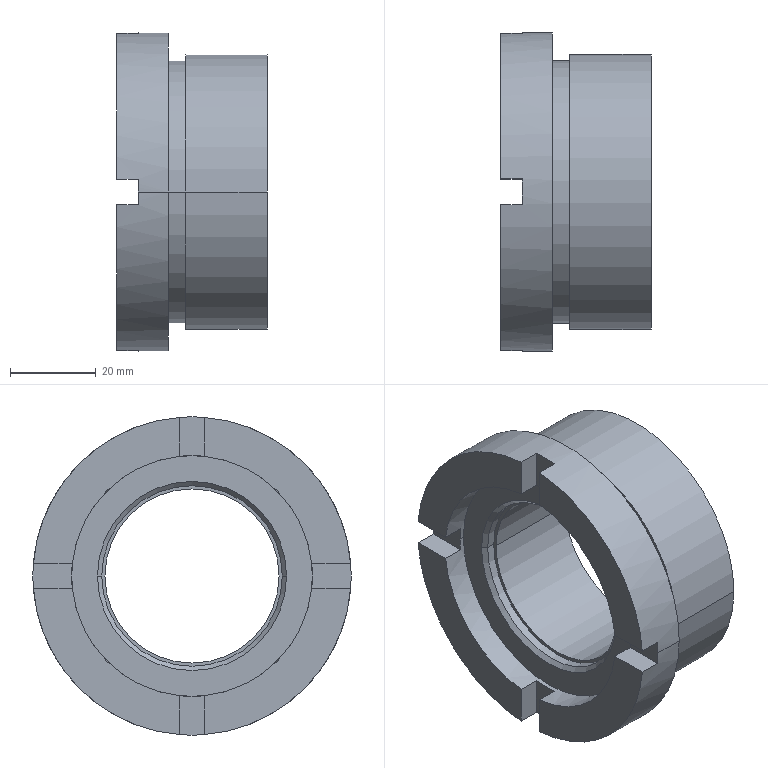Part | SolidWorks | features CirPattern 1, ICE 1, Revolution 1 | 1 solid | 37 faces | box 35 x 74 x 74 mm | volume 68562 mm3 | plane 21 | cylinder 12 | cone 4 | commonest cylinder face diameters 40.5 x2 42 x2 56 x2 61 x2 64 x2 74 x2
STEP:
#1=CARTESIAN_POINT('',(-3.367,-20.25,0.));
#2=VERTEX_POINT('',#1);
#3=CARTESIAN_POINT('',(-3.367,20.25,0.));
#4=VERTEX_POINT('',#3);
#5=CARTESIAN_POINT('',(-3.367,0.,0.));
#6=DIRECTION('',(1.,0.,0.));
#7=DIRECTION('',(0.,1.,0.));
#8=AXIS2_PLACEMENT_3D('',#5,#6,#7);
#9=CIRCLE('',#8,20.25);
#10=EDGE_CURVE('',#2,#4,#9,.T.);
#11=ORIENTED_EDGE('',*,*,#10,.F.);
#12=CARTESIAN_POINT('',(0.,-29.5,0.));
#13=VERTEX_POINT('',#12);
#14=CARTESIAN_POINT('',(0.,-29.5,0.));
#15=DIRECTION('',(0.342,-0.9397,0.));
#16=VECTOR('',#15,1000.);
#17=LINE('',#14,#16);
#18=EDGE_CURVE('',#2,#13,#17,.T.);
#19=ORIENTED_EDGE('',*,*,#18,.T.);
#20=CARTESIAN_POINT('',(0.,29.5,0.));
#21=VERTEX_POINT('',#20);
#22=CARTESIAN_POINT('',(0.,0.,0.));
#23=DIRECTION('',(1.,0.,0.));
#24=DIRECTION('',(0.,1.,0.));
#25=AXIS2_PLACEMENT_3D('',#22,#23,#24);
#26=CIRCLE('',#25,29.5);
#27=EDGE_CURVE('',#13,#21,#26,.T.);
#28=ORIENTED_EDGE('',*,*,#27,.T.);
#29=CARTESIAN_POINT('',(0.,29.5,0.));
#30=DIRECTION('',(0.342,0.9397,0.));
#31=VECTOR('',#30,1000.);
#32=LINE('',#29,#31);
#33=EDGE_CURVE('',#4,#21,#32,.T.);
#34=ORIENTED_EDGE('',*,*,#33,.F.);
#35=EDGE_LOOP('',(#11,#19,#28,#34));
#36=FACE_OUTER_BOUND('',#35,.T.);
#37=CARTESIAN_POINT('',(0.,0.,0.));
#38=DIRECTION('',(1.,0.,0.));
#39=DIRECTION('',(0.,1.,0.));
#40=AXIS2_PLACEMENT_3D('',#37,#38,#39);
#41=CONICAL_SURFACE('',#40,29.5,1.222);
#42=ADVANCED_FACE('',(#36),#41,.F.);
#43=CARTESIAN_POINT('',(-26.,-20.25,0.));
#44=VERTEX_POINT('',#43);
#45=CARTESIAN_POINT('',(-26.,20.25,0.));
#46=VERTEX_POINT('',#45);
#47=CARTESIAN_POINT('',(-26.,0.,0.));
#48=DIRECTION('',(1.,0.,0.));
#49=DIRECTION('',(0.,1.,0.));
#50=AXIS2_PLACEMENT_3D('',#47,#48,#49);
#51=CIRCLE('',#50,20.25);
#52=EDGE_CURVE('',#44,#46,#51,.T.);
#53=ORIENTED_EDGE('',*,*,#52,.F.);
#54=CARTESIAN_POINT('',(0.,-20.25,0.));
#55=DIRECTION('',(1.,0.,0.));
#56=VECTOR('',#55,1000.);
#57=LINE('',#54,#56);
#58=EDGE_CURVE('',#44,#2,#57,.T.);
#59=ORIENTED_EDGE('',*,*,#58,.T.);
#60=ORIENTED_EDGE('',*,*,#10,.T.);
#61=CARTESIAN_POINT('',(0.,20.25,0.));
#62=DIRECTION('',(1.,0.,0.));
#63=VECTOR('',#62,1000.);
#64=LINE('',#61,#63);
#65=EDGE_CURVE('',#46,#4,#64,.T.);
#66=ORIENTED_EDGE('',*,*,#65,.F.);
#67=EDGE_LOOP('',(#53,#59,#60,#66));
#68=FACE_OUTER_BOUND('',#67,.T.);
#69=CARTESIAN_POINT('',(0.,0.,0.));
#70=DIRECTION('',(1.,0.,0.));
#71=DIRECTION('',(0.,1.,0.));
#72=AXIS2_PLACEMENT_3D('',#69,#70,#71);
#73=CYLINDRICAL_SURFACE('',#72,20.25);
#74=ADVANCED_FACE('',(#68),#73,.F.);
#75=CARTESIAN_POINT('',(-28.,-21.,0.));
#76=VERTEX_POINT('',#75);
#77=CARTESIAN_POINT('',(-28.,21.,0.));
#78=VERTEX_POINT('',#77);
#79=CARTESIAN_POINT('',(-28.,0.,0.));
#80=DIRECTION('',(1.,0.,0.));
#81=DIRECTION('',(0.,1.,0.));
#82=AXIS2_PLACEMENT_3D('',#79,#80,#81);
#83=CIRCLE('',#82,21.);
#84=EDGE_CURVE('',#76,#78,#83,.T.);
#85=ORIENTED_EDGE('',*,*,#84,.F.);
#86=CARTESIAN_POINT('',(-26.,-21.,0.));
#87=VERTEX_POINT('',#86);
#88=CARTESIAN_POINT('',(0.,-21.,0.));
#89=DIRECTION('',(1.,0.,0.));
#90=VECTOR('',#89,1000.);
#91=LINE('',#88,#90);
#92=EDGE_CURVE('',#76,#87,#91,.T.);
#93=ORIENTED_EDGE('',*,*,#92,.T.);
#94=CARTESIAN_POINT('',(-26.,21.,0.));
#95=VERTEX_POINT('',#94);
#96=CARTESIAN_POINT('',(-26.,0.,0.));
#97=DIRECTION('',(1.,0.,0.));
#98=DIRECTION('',(0.,1.,0.));
#99=AXIS2_PLACEMENT_3D('',#96,#97,#98);
#100=CIRCLE('',#99,21.);
#101=EDGE_CURVE('',#87,#95,#100,.T.);
#102=ORIENTED_EDGE('',*,*,#101,.T.);
#103=CARTESIAN_POINT('',(0.,21.,0.));
#104=DIRECTION('',(1.,0.,0.));
#105=VECTOR('',#104,1000.);
#106=LINE('',#103,#105);
#107=EDGE_CURVE('',#78,#95,#106,.T.);
#108=ORIENTED_EDGE('',*,*,#107,.F.);
#109=EDGE_LOOP('',(#85,#93,#102,#108));
#110=FACE_OUTER_BOUND('',#109,.T.);
#111=CARTESIAN_POINT('',(0.,0.,0.));
#112=DIRECTION('',(1.,0.,0.));
#113=DIRECTION('',(0.,1.,0.));
#114=AXIS2_PLACEMENT_3D('',#111,#112,#113);
#115=CYLINDRICAL_SURFACE('',#114,21.);
#116=ADVANCED_FACE('',(#110),#115,.F.);
#117=ORIENTED_EDGE('',*,*,#84,.T.);
#118=CARTESIAN_POINT('',(-29.,22.,0.));
#119=VERTEX_POINT('',#118);
#120=CARTESIAN_POINT('',(-28.,21.,0.));
#121=DIRECTION('',(-0.7071,0.7071,0.));
#122=VECTOR('',#121,1000.);
#123=LINE('',#120,#122);
#124=EDGE_CURVE('',#78,#119,#123,.T.);
#125=ORIENTED_EDGE('',*,*,#124,.T.);
#126=CARTESIAN_POINT('',(-29.,-22.,0.));
#127=VERTEX_POINT('',#126);
#128=CARTESIAN_POINT('',(-29.,0.,0.));
#129=DIRECTION('',(1.,0.,0.));
#130=DIRECTION('',(0.,1.,0.));
#131=AXIS2_PLACEMENT_3D('',#128,#129,#130);
#132=CIRCLE('',#131,22.);
#133=EDGE_CURVE('',#127,#119,#132,.T.);
#134=ORIENTED_EDGE('',*,*,#133,.F.);
#135=CARTESIAN_POINT('',(-28.,-21.,0.));
#136=DIRECTION('',(-0.7071,-0.7071,0.));
#137=VECTOR('',#136,1000.);
#138=LINE('',#135,#137);
#139=EDGE_CURVE('',#76,#127,#138,.T.);
#140=ORIENTED_EDGE('',*,*,#139,.F.);
#141=EDGE_LOOP('',(#117,#125,#134,#140));
#142=FACE_OUTER_BOUND('',#141,.T.);
#143=CARTESIAN_POINT('',(-28.,0.,0.));
#144=DIRECTION('',(-1.,0.,0.));
#145=DIRECTION('',(0.,-1.,0.));
#146=AXIS2_PLACEMENT_3D('',#143,#144,#145);
#147=CONICAL_SURFACE('',#146,21.,0.7854);
#148=ADVANCED_FACE('',(#142),#147,.F.);
#149=CARTESIAN_POINT('',(-23.,30.5,0.));
#150=VERTEX_POINT('',#149);
#151=CARTESIAN_POINT('',(-23.,-30.5,0.));
#152=VERTEX_POINT('',#151);
#153=CARTESIAN_POINT('',(-23.,0.,0.));
#154=DIRECTION('',(1.,0.,0.));
#155=DIRECTION('',(0.,1.,0.));
#156=AXIS2_PLACEMENT_3D('',#153,#154,#155);
#157=CIRCLE('',#156,30.5);
#158=EDGE_CURVE('',#150,#152,#157,.T.);
#159=ORIENTED_EDGE('',*,*,#158,.T.);
#160=CARTESIAN_POINT('',(-19.,-30.5,0.));
#161=VERTEX_POINT('',#160);
#162=CARTESIAN_POINT('',(0.,-30.5,0.));
#163=DIRECTION('',(1.,0.,0.));
#164=VECTOR('',#163,1000.);
#165=LINE('',#162,#164);
#166=EDGE_CURVE('',#152,#161,#165,.T.);
#167=ORIENTED_EDGE('',*,*,#166,.T.);
#168=CARTESIAN_POINT('',(-19.,30.5,0.));
#169=VERTEX_POINT('',#168);
#170=CARTESIAN_POINT('',(-19.,0.,0.));
#171=DIRECTION('',(1.,0.,0.));
#172=DIRECTION('',(0.,1.,0.));
#173=AXIS2_PLACEMENT_3D('',#170,#171,#172);
#174=CIRCLE('',#173,30.5);
#175=EDGE_CURVE('',#169,#161,#174,.T.);
#176=ORIENTED_EDGE('',*,*,#175,.F.);
#177=CARTESIAN_POINT('',(0.,30.5,0.));
#178=DIRECTION('',(1.,0.,0.));
#179=VECTOR('',#178,1000.);
#180=LINE('',#177,#179);
#181=EDGE_CURVE('',#150,#169,#180,.T.);
#182=ORIENTED_EDGE('',*,*,#181,.F.);
#183=EDGE_LOOP('',(#159,#167,#176,#182));
#184=FACE_OUTER_BOUND('',#183,.T.);
#185=CARTESIAN_POINT('',(0.,0.,0.));
#186=DIRECTION('',(1.,0.,0.));
#187=DIRECTION('',(0.,1.,0.));
#188=AXIS2_PLACEMENT_3D('',#185,#186,#187);
#189=CYLINDRICAL_SURFACE('',#188,30.5);
#190=ADVANCED_FACE('',(#184),#189,.T.);
#191=CARTESIAN_POINT('',(-19.,32.,0.));
#192=VERTEX_POINT('',#191);
#193=CARTESIAN_POINT('',(-19.,-32.,0.));
#194=VERTEX_POINT('',#193);
#195=CARTESIAN_POINT('',(-19.,0.,0.));
#196=DIRECTION('',(1.,0.,0.));
#197=DIRECTION('',(0.,1.,0.));
#198=AXIS2_PLACEMENT_3D('',#195,#196,#197);
#199=CIRCLE('',#198,32.);
#200=EDGE_CURVE('',#192,#194,#199,.T.);
#201=ORIENTED_EDGE('',*,*,#200,.T.);
#202=CARTESIAN_POINT('',(0.,-32.,0.));
#203=VERTEX_POINT('',#202);
#204=CARTESIAN_POINT('',(0.,-32.,0.));
#205=DIRECTION('',(1.,0.,0.));
#206=VECTOR('',#205,1000.);
#207=LINE('',#204,#206);
#208=EDGE_CURVE('',#194,#203,#207,.T.);
#209=ORIENTED_EDGE('',*,*,#208,.T.);
#210=CARTESIAN_POINT('',(0.,32.,0.));
#211=VERTEX_POINT('',#210);
#212=CARTESIAN_POINT('',(0.,0.,0.));
#213=DIRECTION('',(1.,0.,0.));
#214=DIRECTION('',(0.,1.,0.));
#215=AXIS2_PLACEMENT_3D('',#212,#213,#214);
#216=CIRCLE('',#215,32.);
#217=EDGE_CURVE('',#211,#203,#216,.T.);
#218=ORIENTED_EDGE('',*,*,#217,.F.);
#219=CARTESIAN_POINT('',(0.,32.,0.));
#220=DIRECTION('',(1.,0.,0.));
#221=VECTOR('',#220,1000.);
#222=LINE('',#219,#221);
#223=EDGE_CURVE('',#192,#211,#222,.T.);
#224=ORIENTED_EDGE('',*,*,#223,.F.);
#225=EDGE_LOOP('',(#201,#209,#218,#224));
#226=FACE_OUTER_BOUND('',#225,.T.);
#227=CARTESIAN_POINT('',(0.,0.,0.));
#228=DIRECTION('',(1.,0.,0.));
#229=DIRECTION('',(0.,1.,0.));
#230=AXIS2_PLACEMENT_3D('',#227,#228,#229);
#231=CYLINDRICAL_SURFACE('',#230,32.);
#232=ADVANCED_FACE('',(#226),#231,.T.);
#233=CARTESIAN_POINT('',(-30.,-28.,0.));
#234=VERTEX_POINT('',#233);
#235=CARTESIAN_POINT('',(-30.,-27.839,-3.));
#236=VERTEX_POINT('',#235);
#237=CARTESIAN_POINT('',(-30.,0.,0.));
#238=DIRECTION('',(1.,0.,0.));
#239=DIRECTION('',(0.,1.,0.));
#240=AXIS2_PLACEMENT_3D('',#237,#238,#239);
#241=CIRCLE('',#240,28.);
#242=EDGE_CURVE('',#234,#236,#241,.T.);
#243=ORIENTED_EDGE('',*,*,#242,.F.);
#244=CARTESIAN_POINT('',(-29.,-28.,0.));
#245=VERTEX_POINT('',#244);
#246=CARTESIAN_POINT('',(0.,-28.,0.));
#247=DIRECTION('',(1.,0.,0.));
#248=VECTOR('',#247,1000.);
#249=LINE('',#246,#248);
#250=EDGE_CURVE('',#234,#245,#249,.T.);
#251=ORIENTED_EDGE('',*,*,#250,.T.);
#252=CARTESIAN_POINT('',(-29.,28.,0.));
#253=VERTEX_POINT('',#252);
#254=CARTESIAN_POINT('',(-29.,0.,0.));
#255=DIRECTION('',(1.,0.,0.));
#256=DIRECTION('',(0.,1.,0.));
#257=AXIS2_PLACEMENT_3D('',#254,#255,#256);
#258=CIRCLE('',#257,28.);
#259=EDGE_CURVE('',#245,#253,#258,.T.);
#260=ORIENTED_EDGE('',*,*,#259,.T.);
#261=CARTESIAN_POINT('',(-30.,28.,0.));
#262=VERTEX_POINT('',#261);
#263=CARTESIAN_POINT('',(0.,28.,0.));
#264=DIRECTION('',(1.,0.,0.));
#265=VECTOR('',#264,1000.);
#266=LINE('',#263,#265);
#267=EDGE_CURVE('',#262,#253,#266,.T.);
#268=ORIENTED_EDGE('',*,*,#267,.F.);
#269=CARTESIAN_POINT('',(-30.,27.839,-3.));
#270=VERTEX_POINT('',#269);
#271=CARTESIAN_POINT('',(-30.,0.,0.));
#272=DIRECTION('',(1.,0.,0.));
#273=DIRECTION('',(0.,-1.,0.));
#274=AXIS2_PLACEMENT_3D('',#271,#272,#273);
#275=CIRCLE('',#274,28.);
#276=EDGE_CURVE('',#270,#262,#275,.T.);
#277=ORIENTED_EDGE('',*,*,#276,.F.);
#278=CARTESIAN_POINT('',(-35.,27.839,-3.));
#279=VERTEX_POINT('',#278);
#280=CARTESIAN_POINT('',(-30.,27.839,-3.));
#281=DIRECTION('',(-1.,0.,0.));
#282=VECTOR('',#281,1000.);
#283=LINE('',#280,#282);
#284=EDGE_CURVE('',#270,#279,#283,.T.);
#285=ORIENTED_EDGE('',*,*,#284,.T.);
#286=CARTESIAN_POINT('',(-35.,3.,-27.839));
#287=VERTEX_POINT('',#286);
#288=CARTESIAN_POINT('',(-35.,0.,0.));
#289=DIRECTION('',(1.,0.,0.));
#290=DIRECTION('',(0.,1.,0.));
#291=AXIS2_PLACEMENT_3D('',#288,#289,#290);
#292=CIRCLE('',#291,28.);
#293=EDGE_CURVE('',#287,#279,#292,.T.);
#294=ORIENTED_EDGE('',*,*,#293,.F.);
#295=CARTESIAN_POINT('',(-30.,3.,-27.839));
#296=VERTEX_POINT('',#295);
#297=CARTESIAN_POINT('',(-30.,3.,-27.839));
#298=DIRECTION('',(-1.,0.,0.));
#299=VECTOR('',#298,1000.);
#300=LINE('',#297,#299);
#301=EDGE_CURVE('',#296,#287,#300,.T.);
#302=ORIENTED_EDGE('',*,*,#301,.F.);
#303=CARTESIAN_POINT('',(-30.,-3.,-27.839));
#304=VERTEX_POINT('',#303);
#305=CARTESIAN_POINT('',(-30.,0.,0.));
#306=DIRECTION('',(1.,0.,0.));
#307=DIRECTION('',(0.,0.,1.));
#308=AXIS2_PLACEMENT_3D('',#305,#306,#307);
#309=CIRCLE('',#308,28.);
#310=EDGE_CURVE('',#304,#296,#309,.T.);
#311=ORIENTED_EDGE('',*,*,#310,.F.);
#312=CARTESIAN_POINT('',(-35.,-3.,-27.839));
#313=VERTEX_POINT('',#312);
#314=CARTESIAN_POINT('',(-30.,-3.,-27.839));
#315=DIRECTION('',(-1.,0.,0.));
#316=VECTOR('',#315,1000.);
#317=LINE('',#314,#316);
#318=EDGE_CURVE('',#304,#313,#317,.T.);
#319=ORIENTED_EDGE('',*,*,#318,.T.);
#320=CARTESIAN_POINT('',(-35.,-27.839,-3.));
#321=VERTEX_POINT('',#320);
#322=CARTESIAN_POINT('',(-35.,0.,0.));
#323=DIRECTION('',(1.,0.,0.));
#324=DIRECTION('',(0.,1.,0.));
#325=AXIS2_PLACEMENT_3D('',#322,#323,#324);
#326=CIRCLE('',#325,28.);
#327=EDGE_CURVE('',#321,#313,#326,.T.);
#328=ORIENTED_EDGE('',*,*,#327,.F.);
#329=CARTESIAN_POINT('',(-30.,-27.839,-3.));
#330=DIRECTION('',(-1.,0.,0.));
#331=VECTOR('',#330,1000.);
#332=LINE('',#329,#331);
#333=EDGE_CURVE('',#236,#321,#332,.T.);
#334=ORIENTED_EDGE('',*,*,#333,.F.);
#335=EDGE_LOOP('',(#243,#251,#260,#268,#277,#285,#294,#302,#311,#319,#328,#334));
#336=FACE_OUTER_BOUND('',#335,.T.);
#337=CARTESIAN_POINT('',(0.,0.,0.));
#338=DIRECTION('',(1.,0.,0.));
#339=DIRECTION('',(0.,1.,0.));
#340=AXIS2_PLACEMENT_3D('',#337,#338,#339);
#341=CYLINDRICAL_SURFACE('',#340,28.);
#342=ADVANCED_FACE('',(#336),#341,.F.);
#343=CARTESIAN_POINT('',(-30.,-37.,0.));
#344=VERTEX_POINT('',#343);
#345=CARTESIAN_POINT('',(-30.,-36.878,3.));
#346=VERTEX_POINT('',#345);
#347=CARTESIAN_POINT('',(-30.,0.,0.));
#348=DIRECTION('',(-1.,0.,0.));
#349=DIRECTION('',(0.,1.,0.));
#350=AXIS2_PLACEMENT_3D('',#347,#348,#349);
#351=CIRCLE('',#350,37.);
#352=EDGE_CURVE('',#344,#346,#351,.T.);
#353=ORIENTED_EDGE('',*,*,#352,.F.);
#354=CARTESIAN_POINT('',(-23.,-37.,0.));
#355=VERTEX_POINT('',#354);
#356=CARTESIAN_POINT('',(0.,-37.,0.));
#357=DIRECTION('',(1.,0.,0.));
#358=VECTOR('',#357,1000.);
#359=LINE('',#356,#358);
#360=EDGE_CURVE('',#344,#355,#359,.T.);
#361=ORIENTED_EDGE('',*,*,#360,.T.);
#362=CARTESIAN_POINT('',(-23.,37.,0.));
#363=VERTEX_POINT('',#362);
#364=CARTESIAN_POINT('',(-23.,0.,0.));
#365=DIRECTION('',(1.,0.,0.));
#366=DIRECTION('',(0.,1.,0.));
#367=AXIS2_PLACEMENT_3D('',#364,#365,#366);
#368=CIRCLE('',#367,37.);
#369=EDGE_CURVE('',#363,#355,#368,.T.);
#370=ORIENTED_EDGE('',*,*,#369,.F.);
#371=CARTESIAN_POINT('',(-30.,37.,0.));
#372=VERTEX_POINT('',#371);
#373=CARTESIAN_POINT('',(0.,37.,0.));
#374=DIRECTION('',(1.,0.,0.));
#375=VECTOR('',#374,1000.);
#376=LINE('',#373,#375);
#377=EDGE_CURVE('',#372,#363,#376,.T.);
#378=ORIENTED_EDGE('',*,*,#377,.F.);
#379=CARTESIAN_POINT('',(-30.,36.878,3.));
#380=VERTEX_POINT('',#379);
#381=CARTESIAN_POINT('',(-30.,0.,0.));
#382=DIRECTION('',(-1.,0.,0.));
#383=DIRECTION('',(0.,-1.,0.));
#384=AXIS2_PLACEMENT_3D('',#381,#382,#383);
#385=CIRCLE('',#384,37.);
#386=EDGE_CURVE('',#380,#372,#385,.T.);
#387=ORIENTED_EDGE('',*,*,#386,.F.);
#388=CARTESIAN_POINT('',(-35.,36.878,3.));
#389=VERTEX_POINT('',#388);
#390=CARTESIAN_POINT('',(-30.,36.878,3.));
#391=DIRECTION('',(-1.,0.,0.));
#392=VECTOR('',#391,1000.);
#393=LINE('',#390,#392);
#394=EDGE_CURVE('',#380,#389,#393,.T.);
#395=ORIENTED_EDGE('',*,*,#394,.T.);
#396=CARTESIAN_POINT('',(-35.,3.,36.878));
#397=VERTEX_POINT('',#396);
#398=CARTESIAN_POINT('',(-35.,0.,0.));
#399=DIRECTION('',(1.,0.,0.));
#400=DIRECTION('',(0.,1.,0.));
#401=AXIS2_PLACEMENT_3D('',#398,#399,#400);
#402=CIRCLE('',#401,37.);
#403=EDGE_CURVE('',#389,#397,#402,.T.);
#404=ORIENTED_EDGE('',*,*,#403,.T.);
#405=CARTESIAN_POINT('',(-30.,3.,36.878));
#406=VERTEX_POINT('',#405);
#407=CARTESIAN_POINT('',(-30.,3.,36.878));
#408=DIRECTION('',(-1.,0.,0.));
#409=VECTOR('',#408,1000.);
#410=LINE('',#407,#409);
#411=EDGE_CURVE('',#406,#397,#410,.T.);
#412=ORIENTED_EDGE('',*,*,#411,.F.);
#413=CARTESIAN_POINT('',(-30.,-3.,36.878));
#414=VERTEX_POINT('',#413);
#415=CARTESIAN_POINT('',(-30.,0.,0.));
#416=DIRECTION('',(-1.,0.,0.));
#417=DIRECTION('',(0.,0.,-1.));
#418=AXIS2_PLACEMENT_3D('',#415,#416,#417);
#419=CIRCLE('',#418,37.);
#420=EDGE_CURVE('',#414,#406,#419,.T.);
#421=ORIENTED_EDGE('',*,*,#420,.F.);
#422=CARTESIAN_POINT('',(-35.,-3.,36.878));
#423=VERTEX_POINT('',#422);
#424=CARTESIAN_POINT('',(-30.,-3.,36.878));
#425=DIRECTION('',(-1.,0.,0.));
#426=VECTOR('',#425,1000.);
#427=LINE('',#424,#426);
#428=EDGE_CURVE('',#414,#423,#427,.T.);
#429=ORIENTED_EDGE('',*,*,#428,.T.);
#430=CARTESIAN_POINT('',(-35.,-36.878,3.));
#431=VERTEX_POINT('',#430);
#432=CARTESIAN_POINT('',(-35.,0.,0.));
#433=DIRECTION('',(1.,0.,0.));
#434=DIRECTION('',(0.,1.,0.));
#435=AXIS2_PLACEMENT_3D('',#432,#433,#434);
#436=CIRCLE('',#435,37.);
#437=EDGE_CURVE('',#423,#431,#436,.T.);
#438=ORIENTED_EDGE('',*,*,#437,.T.);
#439=CARTESIAN_POINT('',(-30.,-36.878,3.));
#440=DIRECTION('',(-1.,0.,0.));
#441=VECTOR('',#440,1000.);
#442=LINE('',#439,#441);
#443=EDGE_CURVE('',#346,#431,#442,.T.);
#444=ORIENTED_EDGE('',*,*,#443,.F.);
#445=EDGE_LOOP('',(#353,#361,#370,#378,#387,#395,#404,#412,#421,#429,#438,#444));
#446=FACE_OUTER_BOUND('',#445,.T.);
#447=CARTESIAN_POINT('',(0.,0.,0.));
#448=DIRECTION('',(1.,0.,0.));
#449=DIRECTION('',(0.,1.,0.));
#450=AXIS2_PLACEMENT_3D('',#447,#448,#449);
#451=CYLINDRICAL_SURFACE('',#450,37.);
#452=ADVANCED_FACE('',(#446),#451,.T.);
#453=ORIENTED_EDGE('',*,*,#360,.F.);
#454=CARTESIAN_POINT('',(-30.,-36.878,-3.));
#455=VERTEX_POINT('',#454);
#456=CARTESIAN_POINT('',(-30.,0.,0.));
#457=DIRECTION('',(-1.,0.,0.));
#458=DIRECTION('',(0.,1.,0.));
#459=AXIS2_PLACEMENT_3D('',#456,#457,#458);
#460=CIRCLE('',#459,37.);
#461=EDGE_CURVE('',#455,#344,#460,.T.);
#462=ORIENTED_EDGE('',*,*,#461,.F.);
#463=CARTESIAN_POINT('',(-35.,-36.878,-3.));
#464=VERTEX_POINT('',#463);
#465=CARTESIAN_POINT('',(-30.,-36.878,-3.));
#466=DIRECTION('',(-1.,0.,0.));
#467=VECTOR('',#466,1000.);
#468=LINE('',#465,#467);
#469=EDGE_CURVE('',#455,#464,#468,.T.);
#470=ORIENTED_EDGE('',*,*,#469,.T.);
#471=CARTESIAN_POINT('',(-35.,-3.,-36.878));
#472=VERTEX_POINT('',#471);
#473=CARTESIAN_POINT('',(-35.,0.,0.));
#474=DIRECTION('',(1.,0.,0.));
#475=DIRECTION('',(0.,1.,0.));
#476=AXIS2_PLACEMENT_3D('',#473,#474,#475);
#477=CIRCLE('',#476,37.);
#478=EDGE_CURVE('',#464,#472,#477,.T.);
#479=ORIENTED_EDGE('',*,*,#478,.T.);
#480=CARTESIAN_POINT('',(-30.,-3.,-36.878));
#481=VERTEX_POINT('',#480);
#482=CARTESIAN_POINT('',(-30.,-3.,-36.878));
#483=DIRECTION('',(-1.,0.,0.));
#484=VECTOR('',#483,1000.);
#485=LINE('',#482,#484);
#486=EDGE_CURVE('',#481,#472,#485,.T.);
#487=ORIENTED_EDGE('',*,*,#486,.F.);
#488=CARTESIAN_POINT('',(-30.,3.,-36.878));
#489=VERTEX_POINT('',#488);
#490=CARTESIAN_POINT('',(-30.,0.,0.));
#491=DIRECTION('',(-1.,0.,0.));
#492=DIRECTION('',(0.,0.,1.));
#493=AXIS2_PLACEMENT_3D('',#490,#491,#492);
#494=CIRCLE('',#493,37.);
#495=EDGE_CURVE('',#489,#481,#494,.T.);
#496=ORIENTED_EDGE('',*,*,#495,.F.);
#497=CARTESIAN_POINT('',(-35.,3.,-36.878));
#498=VERTEX_POINT('',#497);
#499=CARTESIAN_POINT('',(-30.,3.,-36.878));
#500=DIRECTION('',(-1.,0.,0.));
#501=VECTOR('',#500,1000.);
#502=LINE('',#499,#501);
#503=EDGE_CURVE('',#489,#498,#502,.T.);
#504=ORIENTED_EDGE('',*,*,#503,.T.);
#505=CARTESIAN_POINT('',(-35.,36.878,-3.));
#506=VERTEX_POINT('',#505);
#507=CARTESIAN_POINT('',(-35.,0.,0.));
#508=DIRECTION('',(1.,0.,0.));
#509=DIRECTION('',(0.,1.,0.));
#510=AXIS2_PLACEMENT_3D('',#507,#508,#509);
#511=CIRCLE('',#510,37.);
#512=EDGE_CURVE('',#498,#506,#511,.T.);
#513=ORIENTED_EDGE('',*,*,#512,.T.);
#514=CARTESIAN_POINT('',(-30.,36.878,-3.));
#515=VERTEX_POINT('',#514);
#516=CARTESIAN_POINT('',(-30.,36.878,-3.));
#517=DIRECTION('',(-1.,0.,0.));
#518=VECTOR('',#517,1000.);
#519=LINE('',#516,#518);
#520=EDGE_CURVE('',#515,#506,#519,.T.);
#521=ORIENTED_EDGE('',*,*,#520,.F.);
#522=CARTESIAN_POINT('',(-30.,0.,0.));
#523=DIRECTION('',(-1.,0.,0.));
#524=DIRECTION('',(0.,-1.,0.));
#525=AXIS2_PLACEMENT_3D('',#522,#523,#524);
#526=CIRCLE('',#525,37.);
#527=EDGE_CURVE('',#372,#515,#526,.T.);
#528=ORIENTED_EDGE('',*,*,#527,.F.);
#529=ORIENTED_EDGE('',*,*,#377,.T.);
#530=CARTESIAN_POINT('',(-23.,0.,0.));
#531=DIRECTION('',(1.,0.,0.));
#532=DIRECTION('',(0.,1.,0.));
#533=AXIS2_PLACEMENT_3D('',#530,#531,#532);
#534=CIRCLE('',#533,37.);
#535=EDGE_CURVE('',#355,#363,#534,.T.);
#536=ORIENTED_EDGE('',*,*,#535,.F.);
#537=EDGE_LOOP('',(#453,#462,#470,#479,#487,#496,#504,#513,#521,#528,#529,#536));
#538=FACE_OUTER_BOUND('',#537,.T.);
#539=CARTESIAN_POINT('',(0.,0.,0.));
#540=DIRECTION('',(1.,0.,0.));
#541=DIRECTION('',(0.,1.,0.));
#542=AXIS2_PLACEMENT_3D('',#539,#540,#541);
#543=CYLINDRICAL_SURFACE('',#542,37.);
#544=ADVANCED_FACE('',(#538),#543,.T.);
#545=CARTESIAN_POINT('',(-35.,-3.,0.));
#546=DIRECTION('',(0.,0.,-1.));
#547=VECTOR('',#546,1000.);
#548=LINE('',#545,#547);
#549=EDGE_CURVE('',#313,#472,#548,.T.);
#550=ORIENTED_EDGE('',*,*,#549,.T.);
#551=ORIENTED_EDGE('',*,*,#478,.F.);
#552=CARTESIAN_POINT('',(-35.,0.,-3.));
#553=DIRECTION('',(0.,-1.,0.));
#554=VECTOR('',#553,1000.);
#555=LINE('',#552,#554);
#556=EDGE_CURVE('',#321,#464,#555,.T.);
#557=ORIENTED_EDGE('',*,*,#556,.F.);
#558=ORIENTED_EDGE('',*,*,#327,.T.);
#559=EDGE_LOOP('',(#550,#551,#557,#558));
#560=FACE_OUTER_BOUND('',#559,.T.);
#561=CARTESIAN_POINT('',(-35.,0.,0.));
#562=DIRECTION('',(1.,0.,0.));
#563=DIRECTION('',(0.,1.,0.));
#564=AXIS2_PLACEMENT_3D('',#561,#562,#563);
#565=PLANE('',#564);
#566=ADVANCED_FACE('',(#560),#565,.F.);
#567=CARTESIAN_POINT('',(-35.,-27.839,3.));
#568=VERTEX_POINT('',#567);
#569=CARTESIAN_POINT('',(-35.,0.,3.));
#570=DIRECTION('',(0.,-1.,0.));
#571=VECTOR('',#570,1000.);
#572=LINE('',#569,#571);
#573=EDGE_CURVE('',#568,#431,#572,.T.);
#574=ORIENTED_EDGE('',*,*,#573,.T.);
#575=ORIENTED_EDGE('',*,*,#437,.F.);
#576=CARTESIAN_POINT('',(-35.,-3.,27.839));
#577=VERTEX_POINT('',#576);
#578=CARTESIAN_POINT('',(-35.,-3.,0.));
#579=DIRECTION('',(0.,0.,1.));
#580=VECTOR('',#579,1000.);
#581=LINE('',#578,#580);
#582=EDGE_CURVE('',#577,#423,#581,.T.);
#583=ORIENTED_EDGE('',*,*,#582,.F.);
#584=CARTESIAN_POINT('',(-35.,0.,0.));
#585=DIRECTION('',(1.,0.,0.));
#586=DIRECTION('',(0.,1.,0.));
#587=AXIS2_PLACEMENT_3D('',#584,#585,#586);
#588=CIRCLE('',#587,28.);
#589=EDGE_CURVE('',#577,#568,#588,.T.);
#590=ORIENTED_EDGE('',*,*,#589,.T.);
#591=EDGE_LOOP('',(#574,#575,#583,#590));
#592=FACE_OUTER_BOUND('',#591,.T.);
#593=CARTESIAN_POINT('',(-35.,0.,0.));
#594=DIRECTION('',(1.,0.,0.));
#595=DIRECTION('',(0.,1.,0.));
#596=AXIS2_PLACEMENT_3D('',#593,#594,#595);
#597=PLANE('',#596);
#598=ADVANCED_FACE('',(#592),#597,.F.);
#599=CARTESIAN_POINT('',(-35.,3.,27.839));
#600=VERTEX_POINT('',#599);
#601=CARTESIAN_POINT('',(-35.,3.,0.));
#602=DIRECTION('',(0.,0.,1.));
#603=VECTOR('',#602,1000.);
#604=LINE('',#601,#603);
#605=EDGE_CURVE('',#600,#397,#604,.T.);
#606=ORIENTED_EDGE('',*,*,#605,.T.);
#607=ORIENTED_EDGE('',*,*,#403,.F.);
#608=CARTESIAN_POINT('',(-35.,27.839,3.));
#609=VERTEX_POINT('',#608);
#610=CARTESIAN_POINT('',(-35.,0.,3.));
#611=DIRECTION('',(0.,1.,0.));
#612=VECTOR('',#611,1000.);
#613=LINE('',#610,#612);
#614=EDGE_CURVE('',#609,#389,#613,.T.);
#615=ORIENTED_EDGE('',*,*,#614,.F.);
#616=CARTESIAN_POINT('',(-35.,0.,0.));
#617=DIRECTION('',(1.,0.,0.));
#618=DIRECTION('',(0.,1.,0.));
#619=AXIS2_PLACEMENT_3D('',#616,#617,#618);
#620=CIRCLE('',#619,28.);
#621=EDGE_CURVE('',#609,#600,#620,.T.);
#622=ORIENTED_EDGE('',*,*,#621,.T.);
#623=EDGE_LOOP('',(#606,#607,#615,#622));
#624=FACE_OUTER_BOUND('',#623,.T.);
#625=CARTESIAN_POINT('',(-35.,0.,0.));
#626=DIRECTION('',(1.,0.,0.));
#627=DIRECTION('',(0.,1.,0.));
#628=AXIS2_PLACEMENT_3D('',#625,#626,#627);
#629=PLANE('',#628);
#630=ADVANCED_FACE('',(#624),#629,.F.);
#631=ORIENTED_EDGE('',*,*,#250,.F.);
#632=CARTESIAN_POINT('',(-30.,-27.839,3.));
#633=VERTEX_POINT('',#632);
#634=CARTESIAN_POINT('',(-30.,0.,0.));
#635=DIRECTION('',(1.,0.,0.));
#636=DIRECTION('',(0.,1.,0.));
#637=AXIS2_PLACEMENT_3D('',#634,#635,#636);
#638=CIRCLE('',#637,28.);
#639=EDGE_CURVE('',#633,#234,#638,.T.);
#640=ORIENTED_EDGE('',*,*,#639,.F.);
#641=CARTESIAN_POINT('',(-30.,-27.839,3.));
#642=DIRECTION('',(-1.,0.,0.));
#643=VECTOR('',#642,1000.);
#644=LINE('',#641,#643);
#645=EDGE_CURVE('',#633,#568,#644,.T.);
#646=ORIENTED_EDGE('',*,*,#645,.T.);
#647=ORIENTED_EDGE('',*,*,#589,.F.);
#648=CARTESIAN_POINT('',(-30.,-3.,27.839));
#649=VERTEX_POINT('',#648);
#650=CARTESIAN_POINT('',(-30.,-3.,27.839));
#651=DIRECTION('',(-1.,0.,0.));
#652=VECTOR('',#651,1000.);
#653=LINE('',#650,#652);
#654=EDGE_CURVE('',#649,#577,#653,.T.);
#655=ORIENTED_EDGE('',*,*,#654,.F.);
#656=CARTESIAN_POINT('',(-30.,3.,27.839));
#657=VERTEX_POINT('',#656);
#658=CARTESIAN_POINT('',(-30.,0.,0.));
#659=DIRECTION('',(1.,0.,0.));
#660=DIRECTION('',(0.,0.,-1.));
#661=AXIS2_PLACEMENT_3D('',#658,#659,#660);
#662=CIRCLE('',#661,28.);
#663=EDGE_CURVE('',#657,#649,#662,.T.);
#664=ORIENTED_EDGE('',*,*,#663,.F.);
#665=CARTESIAN_POINT('',(-30.,3.,27.839));
#666=DIRECTION('',(-1.,0.,0.));
#667=VECTOR('',#666,1000.);
#668=LINE('',#665,#667);
#669=EDGE_CURVE('',#657,#600,#668,.T.);
#670=ORIENTED_EDGE('',*,*,#669,.T.);
#671=ORIENTED_EDGE('',*,*,#621,.F.);
#672=CARTESIAN_POINT('',(-30.,27.839,3.));
#673=VERTEX_POINT('',#672);
#674=CARTESIAN_POINT('',(-30.,27.839,3.));
#675=DIRECTION('',(-1.,0.,0.));
#676=VECTOR('',#675,1000.);
#677=LINE('',#674,#676);
#678=EDGE_CURVE('',#673,#609,#677,.T.);
#679=ORIENTED_EDGE('',*,*,#678,.F.);
#680=CARTESIAN_POINT('',(-30.,0.,0.));
#681=DIRECTION('',(1.,0.,0.));
#682=DIRECTION('',(0.,-1.,0.));
#683=AXIS2_PLACEMENT_3D('',#680,#681,#682);
#684=CIRCLE('',#683,28.);
#685=EDGE_CURVE('',#262,#673,#684,.T.);
#686=ORIENTED_EDGE('',*,*,#685,.F.);
#687=ORIENTED_EDGE('',*,*,#267,.T.);
#688=CARTESIAN_POINT('',(-29.,0.,0.));
#689=DIRECTION('',(1.,0.,0.));
#690=DIRECTION('',(0.,1.,0.));
#691=AXIS2_PLACEMENT_3D('',#688,#689,#690);
#692=CIRCLE('',#691,28.);
#693=EDGE_CURVE('',#253,#245,#692,.T.);
#694=ORIENTED_EDGE('',*,*,#693,.T.);
#695=EDGE_LOOP('',(#631,#640,#646,#647,#655,#664,#670,#671,#679,#686,#687,#694));
#696=FACE_OUTER_BOUND('',#695,.T.);
#697=CARTESIAN_POINT('',(0.,0.,0.));
#698=DIRECTION('',(1.,0.,0.));
#699=DIRECTION('',(0.,1.,0.));
#700=AXIS2_PLACEMENT_3D('',#697,#698,#699);
#701=CYLINDRICAL_SURFACE('',#700,28.);
#702=ADVANCED_FACE('',(#696),#701,.F.);
#703=ORIENTED_EDGE('',*,*,#512,.F.);
#704=CARTESIAN_POINT('',(-35.,3.,0.));
#705=DIRECTION('',(0.,0.,-1.));
#706=VECTOR('',#705,1000.);
#707=LINE('',#704,#706);
#708=EDGE_CURVE('',#287,#498,#707,.T.);
#709=ORIENTED_EDGE('',*,*,#708,.F.);
#710=ORIENTED_EDGE('',*,*,#293,.T.);
#711=CARTESIAN_POINT('',(-35.,0.,-3.));
#712=DIRECTION('',(0.,1.,0.));
#713=VECTOR('',#712,1000.);
#714=LINE('',#711,#713);
#715=EDGE_CURVE('',#279,#506,#714,.T.);
#716=ORIENTED_EDGE('',*,*,#715,.T.);
#717=EDGE_LOOP('',(#703,#709,#710,#716));
#718=FACE_OUTER_BOUND('',#717,.T.);
#719=CARTESIAN_POINT('',(-35.,0.,0.));
#720=DIRECTION('',(1.,0.,0.));
#721=DIRECTION('',(0.,1.,0.));
#722=AXIS2_PLACEMENT_3D('',#719,#720,#721);
#723=PLANE('',#722);
#724=ADVANCED_FACE('',(#718),#723,.F.);
#725=ORIENTED_EDGE('',*,*,#208,.F.);
#726=CARTESIAN_POINT('',(-19.,0.,0.));
#727=DIRECTION('',(1.,0.,0.));
#728=DIRECTION('',(0.,1.,0.));
#729=AXIS2_PLACEMENT_3D('',#726,#727,#728);
#730=CIRCLE('',#729,32.);
#731=EDGE_CURVE('',#194,#192,#730,.T.);
#732=ORIENTED_EDGE('',*,*,#731,.T.);
#733=ORIENTED_EDGE('',*,*,#223,.T.);
#734=CARTESIAN_POINT('',(0.,0.,0.));
#735=DIRECTION('',(1.,0.,0.));
#736=DIRECTION('',(0.,1.,0.));
#737=AXIS2_PLACEMENT_3D('',#734,#735,#736);
#738=CIRCLE('',#737,32.);
#739=EDGE_CURVE('',#203,#211,#738,.T.);
#740=ORIENTED_EDGE('',*,*,#739,.F.);
#741=EDGE_LOOP('',(#725,#732,#733,#740));
#742=FACE_OUTER_BOUND('',#741,.T.);
#743=CARTESIAN_POINT('',(0.,0.,0.));
#744=DIRECTION('',(1.,0.,0.));
#745=DIRECTION('',(0.,1.,0.));
#746=AXIS2_PLACEMENT_3D('',#743,#744,#745);
#747=CYLINDRICAL_SURFACE('',#746,32.);
#748=ADVANCED_FACE('',(#742),#747,.T.);
#749=ORIENTED_EDGE('',*,*,#175,.T.);
#750=CARTESIAN_POINT('',(-19.,0.,0.));
#751=DIRECTION('',(1.,0.,0.));
#752=DIRECTION('',(0.,1.,0.));
#753=AXIS2_PLACEMENT_3D('',#750,#751,#752);
#754=CIRCLE('',#753,30.5);
#755=EDGE_CURVE('',#161,#169,#754,.T.);
#756=ORIENTED_EDGE('',*,*,#755,.T.);
#757=EDGE_LOOP('',(#749,#756));
#758=FACE_BOUND('',#757,.T.);
#759=ORIENTED_EDGE('',*,*,#200,.F.);
#760=ORIENTED_EDGE('',*,*,#731,.F.);
#761=EDGE_LOOP('',(#759,#760));
#762=FACE_OUTER_BOUND('',#761,.T.);
#763=CARTESIAN_POINT('',(-19.,0.,0.));
#764=DIRECTION('',(-1.,0.,0.));
#765=DIRECTION('',(0.,-1.,0.));
#766=AXIS2_PLACEMENT_3D('',#763,#764,#765);
#767=PLANE('',#766);
#768=ADVANCED_FACE('',(#758,#762),#767,.T.);
#769=ORIENTED_EDGE('',*,*,#166,.F.);
#770=CARTESIAN_POINT('',(-23.,0.,0.));
#771=DIRECTION('',(1.,0.,0.));
#772=DIRECTION('',(0.,1.,0.));
#773=AXIS2_PLACEMENT_3D('',#770,#771,#772);
#774=CIRCLE('',#773,30.5);
#775=EDGE_CURVE('',#152,#150,#774,.T.);
#776=ORIENTED_EDGE('',*,*,#775,.T.);
#777=ORIENTED_EDGE('',*,*,#181,.T.);
#778=ORIENTED_EDGE('',*,*,#755,.F.);
#779=EDGE_LOOP('',(#769,#776,#777,#778));
#780=FACE_OUTER_BOUND('',#779,.T.);
#781=CARTESIAN_POINT('',(0.,0.,0.));
#782=DIRECTION('',(1.,0.,0.));
#783=DIRECTION('',(0.,1.,0.));
#784=AXIS2_PLACEMENT_3D('',#781,#782,#783);
#785=CYLINDRICAL_SURFACE('',#784,30.5);
#786=ADVANCED_FACE('',(#780),#785,.T.);
#787=ORIENTED_EDGE('',*,*,#158,.F.);
#788=ORIENTED_EDGE('',*,*,#775,.F.);
#789=EDGE_LOOP('',(#787,#788));
#790=FACE_BOUND('',#789,.T.);
#791=ORIENTED_EDGE('',*,*,#369,.T.);
#792=ORIENTED_EDGE('',*,*,#535,.T.);
#793=EDGE_LOOP('',(#791,#792));
#794=FACE_OUTER_BOUND('',#793,.T.);
#795=CARTESIAN_POINT('',(-23.,0.,0.));
#796=DIRECTION('',(-1.,0.,0.));
#797=DIRECTION('',(0.,-1.,0.));
#798=AXIS2_PLACEMENT_3D('',#795,#796,#797);
#799=PLANE('',#798);
#800=ADVANCED_FACE('',(#790,#794),#799,.F.);
#801=ORIENTED_EDGE('',*,*,#693,.F.);
#802=ORIENTED_EDGE('',*,*,#259,.F.);
#803=EDGE_LOOP('',(#801,#802));
#804=FACE_OUTER_BOUND('',#803,.T.);
#805=ORIENTED_EDGE('',*,*,#133,.T.);
#806=CARTESIAN_POINT('',(-29.,0.,0.));
#807=DIRECTION('',(1.,0.,0.));
#808=DIRECTION('',(0.,1.,0.));
#809=AXIS2_PLACEMENT_3D('',#806,#807,#808);
#810=CIRCLE('',#809,22.);
#811=EDGE_CURVE('',#119,#127,#810,.T.);
#812=ORIENTED_EDGE('',*,*,#811,.T.);
#813=EDGE_LOOP('',(#805,#812));
#814=FACE_BOUND('',#813,.T.);
#815=CARTESIAN_POINT('',(-29.,0.,0.));
#816=DIRECTION('',(1.,0.,0.));
#817=DIRECTION('',(0.,1.,0.));
#818=AXIS2_PLACEMENT_3D('',#815,#816,#817);
#819=PLANE('',#818);
#820=ADVANCED_FACE('',(#804,#814),#819,.F.);
#821=ORIENTED_EDGE('',*,*,#124,.F.);
#822=CARTESIAN_POINT('',(-28.,0.,0.));
#823=DIRECTION('',(1.,0.,0.));
#824=DIRECTION('',(0.,1.,0.));
#825=AXIS2_PLACEMENT_3D('',#822,#823,#824);
#826=CIRCLE('',#825,21.);
#827=EDGE_CURVE('',#78,#76,#826,.T.);
#828=ORIENTED_EDGE('',*,*,#827,.T.);
#829=ORIENTED_EDGE('',*,*,#139,.T.);
#830=ORIENTED_EDGE('',*,*,#811,.F.);
#831=EDGE_LOOP('',(#821,#828,#829,#830));
#832=FACE_OUTER_BOUND('',#831,.T.);
#833=CARTESIAN_POINT('',(-28.,0.,0.));
#834=DIRECTION('',(-1.,0.,0.));
#835=DIRECTION('',(0.,-1.,0.));
#836=AXIS2_PLACEMENT_3D('',#833,#834,#835);
#837=CONICAL_SURFACE('',#836,21.,0.7854);
#838=ADVANCED_FACE('',(#832),#837,.F.);
#839=ORIENTED_EDGE('',*,*,#92,.F.);
#840=ORIENTED_EDGE('',*,*,#827,.F.);
#841=ORIENTED_EDGE('',*,*,#107,.T.);
#842=CARTESIAN_POINT('',(-26.,0.,0.));
#843=DIRECTION('',(1.,0.,0.));
#844=DIRECTION('',(0.,1.,0.));
#845=AXIS2_PLACEMENT_3D('',#842,#843,#844);
#846=CIRCLE('',#845,21.);
#847=EDGE_CURVE('',#95,#87,#846,.T.);
#848=ORIENTED_EDGE('',*,*,#847,.T.);
#849=EDGE_LOOP('',(#839,#840,#841,#848));
#850=FACE_OUTER_BOUND('',#849,.T.);
#851=CARTESIAN_POINT('',(0.,0.,0.));
#852=DIRECTION('',(1.,0.,0.));
#853=DIRECTION('',(0.,1.,0.));
#854=AXIS2_PLACEMENT_3D('',#851,#852,#853);
#855=CYLINDRICAL_SURFACE('',#854,21.);
#856=ADVANCED_FACE('',(#850),#855,.F.);
#857=ORIENTED_EDGE('',*,*,#847,.F.);
#858=ORIENTED_EDGE('',*,*,#101,.F.);
#859=EDGE_LOOP('',(#857,#858));
#860=FACE_OUTER_BOUND('',#859,.T.);
#861=CARTESIAN_POINT('',(-26.,0.,0.));
#862=DIRECTION('',(1.,0.,0.));
#863=DIRECTION('',(0.,1.,0.));
#864=AXIS2_PLACEMENT_3D('',#861,#862,#863);
#865=CIRCLE('',#864,20.25);
#866=EDGE_CURVE('',#46,#44,#865,.T.);
#867=ORIENTED_EDGE('',*,*,#866,.T.);
#868=ORIENTED_EDGE('',*,*,#52,.T.);
#869=EDGE_LOOP('',(#867,#868));
#870=FACE_BOUND('',#869,.T.);
#871=CARTESIAN_POINT('',(-26.,0.,0.));
#872=DIRECTION('',(1.,0.,0.));
#873=DIRECTION('',(0.,1.,0.));
#874=AXIS2_PLACEMENT_3D('',#871,#872,#873);
#875=PLANE('',#874);
#876=ADVANCED_FACE('',(#860,#870),#875,.F.);
#877=ORIENTED_EDGE('',*,*,#58,.F.);
#878=ORIENTED_EDGE('',*,*,#866,.F.);
#879=ORIENTED_EDGE('',*,*,#65,.T.);
#880=CARTESIAN_POINT('',(-3.367,0.,0.));
#881=DIRECTION('',(1.,0.,0.));
#882=DIRECTION('',(0.,1.,0.));
#883=AXIS2_PLACEMENT_3D('',#880,#881,#882);
#884=CIRCLE('',#883,20.25);
#885=EDGE_CURVE('',#4,#2,#884,.T.);
#886=ORIENTED_EDGE('',*,*,#885,.T.);
#887=EDGE_LOOP('',(#877,#878,#879,#886));
#888=FACE_OUTER_BOUND('',#887,.T.);
#889=CARTESIAN_POINT('',(0.,0.,0.));
#890=DIRECTION('',(1.,0.,0.));
#891=DIRECTION('',(0.,1.,0.));
#892=AXIS2_PLACEMENT_3D('',#889,#890,#891);
#893=CYLINDRICAL_SURFACE('',#892,20.25);
#894=ADVANCED_FACE('',(#888),#893,.F.);
#895=ORIENTED_EDGE('',*,*,#18,.F.);
#896=ORIENTED_EDGE('',*,*,#885,.F.);
#897=ORIENTED_EDGE('',*,*,#33,.T.);
#898=CARTESIAN_POINT('',(0.,0.,0.));
#899=DIRECTION('',(1.,0.,0.));
#900=DIRECTION('',(0.,1.,0.));
#901=AXIS2_PLACEMENT_3D('',#898,#899,#900);
#902=CIRCLE('',#901,29.5);
#903=EDGE_CURVE('',#21,#13,#902,.T.);
#904=ORIENTED_EDGE('',*,*,#903,.T.);
#905=EDGE_LOOP('',(#895,#896,#897,#904));
#906=FACE_OUTER_BOUND('',#905,.T.);
#907=CARTESIAN_POINT('',(0.,0.,0.));
#908=DIRECTION('',(1.,0.,0.));
#909=DIRECTION('',(0.,1.,0.));
#910=AXIS2_PLACEMENT_3D('',#907,#908,#909);
#911=CONICAL_SURFACE('',#910,29.5,1.222);
#912=ADVANCED_FACE('',(#906),#911,.F.);
#913=ORIENTED_EDGE('',*,*,#217,.T.);
#914=ORIENTED_EDGE('',*,*,#739,.T.);
#915=EDGE_LOOP('',(#913,#914));
#916=FACE_OUTER_BOUND('',#915,.T.);
#917=ORIENTED_EDGE('',*,*,#903,.F.);
#918=ORIENTED_EDGE('',*,*,#27,.F.);
#919=EDGE_LOOP('',(#917,#918));
#920=FACE_BOUND('',#919,.T.);
#921=CARTESIAN_POINT('',(0.,0.,0.));
#922=DIRECTION('',(1.,0.,0.));
#923=DIRECTION('',(0.,1.,0.));
#924=AXIS2_PLACEMENT_3D('',#921,#922,#923);
#925=PLANE('',#924);
#926=ADVANCED_FACE('',(#916,#920),#925,.T.);
#927=ORIENTED_EDGE('',*,*,#715,.F.);
#928=ORIENTED_EDGE('',*,*,#284,.F.);
#929=CARTESIAN_POINT('',(-30.,0.,-3.));
#930=DIRECTION('',(0.,1.,0.));
#931=VECTOR('',#930,1000.);
#932=LINE('',#929,#931);
#933=EDGE_CURVE('',#270,#515,#932,.T.);
#934=ORIENTED_EDGE('',*,*,#933,.T.);
#935=ORIENTED_EDGE('',*,*,#520,.T.);
#936=EDGE_LOOP('',(#927,#928,#934,#935));
#937=FACE_OUTER_BOUND('',#936,.T.);
#938=CARTESIAN_POINT('',(-30.,0.,-3.));
#939=DIRECTION('',(0.,0.,1.));
#940=DIRECTION('',(1.,0.,0.));
#941=AXIS2_PLACEMENT_3D('',#938,#939,#940);
#942=PLANE('',#941);
#943=ADVANCED_FACE('',(#937),#942,.T.);
#944=ORIENTED_EDGE('',*,*,#614,.T.);
#945=ORIENTED_EDGE('',*,*,#394,.F.);
#946=CARTESIAN_POINT('',(-30.,0.,3.));
#947=DIRECTION('',(0.,1.,0.));
#948=VECTOR('',#947,1000.);
#949=LINE('',#946,#948);
#950=EDGE_CURVE('',#673,#380,#949,.T.);
#951=ORIENTED_EDGE('',*,*,#950,.F.);
#952=ORIENTED_EDGE('',*,*,#678,.T.);
#953=EDGE_LOOP('',(#944,#945,#951,#952));
#954=FACE_OUTER_BOUND('',#953,.T.);
#955=CARTESIAN_POINT('',(-30.,0.,3.));
#956=DIRECTION('',(0.,0.,1.));
#957=DIRECTION('',(0.,-1.,0.));
#958=AXIS2_PLACEMENT_3D('',#955,#956,#957);
#959=PLANE('',#958);
#960=ADVANCED_FACE('',(#954),#959,.F.);
#961=ORIENTED_EDGE('',*,*,#276,.T.);
#962=ORIENTED_EDGE('',*,*,#685,.T.);
#963=ORIENTED_EDGE('',*,*,#950,.T.);
#964=ORIENTED_EDGE('',*,*,#386,.T.);
#965=ORIENTED_EDGE('',*,*,#527,.T.);
#966=ORIENTED_EDGE('',*,*,#933,.F.);
#967=EDGE_LOOP('',(#961,#962,#963,#964,#965,#966));
#968=FACE_OUTER_BOUND('',#967,.T.);
#969=CARTESIAN_POINT('',(-30.,0.,0.));
#970=DIRECTION('',(-1.,0.,0.));
#971=DIRECTION('',(0.,-1.,0.));
#972=AXIS2_PLACEMENT_3D('',#969,#970,#971);
#973=PLANE('',#972);
#974=ADVANCED_FACE('',(#968),#973,.T.);
#975=ORIENTED_EDGE('',*,*,#605,.F.);
#976=ORIENTED_EDGE('',*,*,#669,.F.);
#977=CARTESIAN_POINT('',(-30.,3.,0.));
#978=DIRECTION('',(0.,0.,1.));
#979=VECTOR('',#978,1000.);
#980=LINE('',#977,#979);
#981=EDGE_CURVE('',#657,#406,#980,.T.);
#982=ORIENTED_EDGE('',*,*,#981,.T.);
#983=ORIENTED_EDGE('',*,*,#411,.T.);
#984=EDGE_LOOP('',(#975,#976,#982,#983));
#985=FACE_OUTER_BOUND('',#984,.T.);
#986=CARTESIAN_POINT('',(-30.,3.,0.));
#987=DIRECTION('',(0.,-1.,0.));
#988=DIRECTION('',(0.,0.,-1.));
#989=AXIS2_PLACEMENT_3D('',#986,#987,#988);
#990=PLANE('',#989);
#991=ADVANCED_FACE('',(#985),#990,.T.);
#992=ORIENTED_EDGE('',*,*,#582,.T.);
#993=ORIENTED_EDGE('',*,*,#428,.F.);
#994=CARTESIAN_POINT('',(-30.,-3.,0.));
#995=DIRECTION('',(0.,0.,1.));
#996=VECTOR('',#995,1000.);
#997=LINE('',#994,#996);
#998=EDGE_CURVE('',#649,#414,#997,.T.);
#999=ORIENTED_EDGE('',*,*,#998,.F.);
#1000=ORIENTED_EDGE('',*,*,#654,.T.);
#1001=EDGE_LOOP('',(#992,#993,#999,#1000));
#1002=FACE_OUTER_BOUND('',#1001,.T.);
#1003=CARTESIAN_POINT('',(-30.,-3.,0.));
#1004=DIRECTION('',(0.,-1.,0.));
#1005=DIRECTION('',(0.,0.,-1.));
#1006=AXIS2_PLACEMENT_3D('',#1003,#1004,#1005);
#1007=PLANE('',#1006);
#1008=ADVANCED_FACE('',(#1002),#1007,.F.);
#1009=ORIENTED_EDGE('',*,*,#663,.T.);
#1010=ORIENTED_EDGE('',*,*,#998,.T.);
#1011=ORIENTED_EDGE('',*,*,#420,.T.);
#1012=ORIENTED_EDGE('',*,*,#981,.F.);
#1013=EDGE_LOOP('',(#1009,#1010,#1011,#1012));
#1014=FACE_OUTER_BOUND('',#1013,.T.);
#1015=CARTESIAN_POINT('',(-30.,0.,0.));
#1016=DIRECTION('',(-1.,0.,0.));
#1017=DIRECTION('',(0.,0.,-1.));
#1018=AXIS2_PLACEMENT_3D('',#1015,#1016,#1017);
#1019=PLANE('',#1018);
#1020=ADVANCED_FACE('',(#1014),#1019,.T.);
#1021=ORIENTED_EDGE('',*,*,#573,.F.);
#1022=ORIENTED_EDGE('',*,*,#645,.F.);
#1023=CARTESIAN_POINT('',(-30.,0.,3.));
#1024=DIRECTION('',(0.,-1.,0.));
#1025=VECTOR('',#1024,1000.);
#1026=LINE('',#1023,#1025);
#1027=EDGE_CURVE('',#633,#346,#1026,.T.);
#1028=ORIENTED_EDGE('',*,*,#1027,.T.);
#1029=ORIENTED_EDGE('',*,*,#443,.T.);
#1030=EDGE_LOOP('',(#1021,#1022,#1028,#1029));
#1031=FACE_OUTER_BOUND('',#1030,.T.);
#1032=CARTESIAN_POINT('',(-30.,0.,3.));
#1033=DIRECTION('',(0.,0.,-1.));
#1034=DIRECTION('',(-1.,0.,0.));
#1035=AXIS2_PLACEMENT_3D('',#1032,#1033,#1034);
#1036=PLANE('',#1035);
#1037=ADVANCED_FACE('',(#1031),#1036,.T.);
#1038=ORIENTED_EDGE('',*,*,#556,.T.);
#1039=ORIENTED_EDGE('',*,*,#469,.F.);
#1040=CARTESIAN_POINT('',(-30.,0.,-3.));
#1041=DIRECTION('',(0.,-1.,0.));
#1042=VECTOR('',#1041,1000.);
#1043=LINE('',#1040,#1042);
#1044=EDGE_CURVE('',#236,#455,#1043,.T.);
#1045=ORIENTED_EDGE('',*,*,#1044,.F.);
#1046=ORIENTED_EDGE('',*,*,#333,.T.);
#1047=EDGE_LOOP('',(#1038,#1039,#1045,#1046));
#1048=FACE_OUTER_BOUND('',#1047,.T.);
#1049=CARTESIAN_POINT('',(-30.,0.,-3.));
#1050=DIRECTION('',(0.,0.,-1.));
#1051=DIRECTION('',(0.,1.,0.));
#1052=AXIS2_PLACEMENT_3D('',#1049,#1050,#1051);
#1053=PLANE('',#1052);
#1054=ADVANCED_FACE('',(#1048),#1053,.F.);
#1055=ORIENTED_EDGE('',*,*,#639,.T.);
#1056=ORIENTED_EDGE('',*,*,#242,.T.);
#1057=ORIENTED_EDGE('',*,*,#1044,.T.);
#1058=ORIENTED_EDGE('',*,*,#461,.T.);
#1059=ORIENTED_EDGE('',*,*,#352,.T.);
#1060=ORIENTED_EDGE('',*,*,#1027,.F.);
#1061=EDGE_LOOP('',(#1055,#1056,#1057,#1058,#1059,#1060));
#1062=FACE_OUTER_BOUND('',#1061,.T.);
#1063=CARTESIAN_POINT('',(-30.,0.,0.));
#1064=DIRECTION('',(-1.,0.,0.));
#1065=DIRECTION('',(0.,1.,0.));
#1066=AXIS2_PLACEMENT_3D('',#1063,#1064,#1065);
#1067=PLANE('',#1066);
#1068=ADVANCED_FACE('',(#1062),#1067,.T.);
#1069=ORIENTED_EDGE('',*,*,#549,.F.);
#1070=ORIENTED_EDGE('',*,*,#318,.F.);
#1071=CARTESIAN_POINT('',(-30.,-3.,0.));
#1072=DIRECTION('',(0.,0.,-1.));
#1073=VECTOR('',#1072,1000.);
#1074=LINE('',#1071,#1073);
#1075=EDGE_CURVE('',#304,#481,#1074,.T.);
#1076=ORIENTED_EDGE('',*,*,#1075,.T.);
#1077=ORIENTED_EDGE('',*,*,#486,.T.);
#1078=EDGE_LOOP('',(#1069,#1070,#1076,#1077));
#1079=FACE_OUTER_BOUND('',#1078,.T.);
#1080=CARTESIAN_POINT('',(-30.,-3.,0.));
#1081=DIRECTION('',(0.,1.,0.));
#1082=DIRECTION('',(0.,0.,1.));
#1083=AXIS2_PLACEMENT_3D('',#1080,#1081,#1082);
#1084=PLANE('',#1083);
#1085=ADVANCED_FACE('',(#1079),#1084,.T.);
#1086=ORIENTED_EDGE('',*,*,#708,.T.);
#1087=ORIENTED_EDGE('',*,*,#503,.F.);
#1088=CARTESIAN_POINT('',(-30.,3.,0.));
#1089=DIRECTION('',(0.,0.,-1.));
#1090=VECTOR('',#1089,1000.);
#1091=LINE('',#1088,#1090);
#1092=EDGE_CURVE('',#296,#489,#1091,.T.);
#1093=ORIENTED_EDGE('',*,*,#1092,.F.);
#1094=ORIENTED_EDGE('',*,*,#301,.T.);
#1095=EDGE_LOOP('',(#1086,#1087,#1093,#1094));
#1096=FACE_OUTER_BOUND('',#1095,.T.);
#1097=CARTESIAN_POINT('',(-30.,3.,0.));
#1098=DIRECTION('',(0.,1.,0.));
#1099=DIRECTION('',(0.,0.,1.));
#1100=AXIS2_PLACEMENT_3D('',#1097,#1098,#1099);
#1101=PLANE('',#1100);
#1102=ADVANCED_FACE('',(#1096),#1101,.F.);
#1103=ORIENTED_EDGE('',*,*,#310,.T.);
#1104=ORIENTED_EDGE('',*,*,#1092,.T.);
#1105=ORIENTED_EDGE('',*,*,#495,.T.);
#1106=ORIENTED_EDGE('',*,*,#1075,.F.);
#1107=EDGE_LOOP('',(#1103,#1104,#1105,#1106));
#1108=FACE_OUTER_BOUND('',#1107,.T.);
#1109=CARTESIAN_POINT('',(-30.,0.,0.));
#1110=DIRECTION('',(-1.,0.,0.));
#1111=DIRECTION('',(0.,0.,1.));
#1112=AXIS2_PLACEMENT_3D('',#1109,#1110,#1111);
#1113=PLANE('',#1112);
#1114=ADVANCED_FACE('',(#1108),#1113,.T.);
#1115=CLOSED_SHELL('',(#42,#74,#116,#148,#190,#232,#342,#452,#544,#566,#598,#630,#702,#724,#748,#768,#786,#800,#820,#838,#856,#876,#894,#912,#926,#943,#960,#974,#991,#1008,#1020,#1037,#1054,#1068,#1085,#1102,#1114));
#1116=MANIFOLD_SOLID_BREP('',#1115);
#1117=CARTESIAN_POINT('',(0.,0.,0.));
#1118=DIRECTION('',(0.,0.,1.));
#1119=DIRECTION('',(1.,0.,0.));
#1120=AXIS2_PLACEMENT_3D('',#1117,#1118,#1119);
#1121=(LENGTH_UNIT()NAMED_UNIT(*)SI_UNIT(.MILLI.,.METRE.));
#1122=UNCERTAINTY_MEASURE_WITH_UNIT(LENGTH_MEASURE(0.00001),#1121,'','');
#1123=(NAMED_UNIT(*)PLANE_ANGLE_UNIT()SI_UNIT($,.RADIAN.));
#1124=(NAMED_UNIT(*)SI_UNIT($,.STERADIAN.)SOLID_ANGLE_UNIT());
#1125=(GEOMETRIC_REPRESENTATION_CONTEXT(3)GLOBAL_UNCERTAINTY_ASSIGNED_CONTEXT((#1122))GLOBAL_UNIT_ASSIGNED_CONTEXT((#1121,#1123,#1124))REPRESENTATION_CONTEXT('',''));
#1126=ADVANCED_BREP_SHAPE_REPRESENTATION('',(#1116,#1120),#1125);